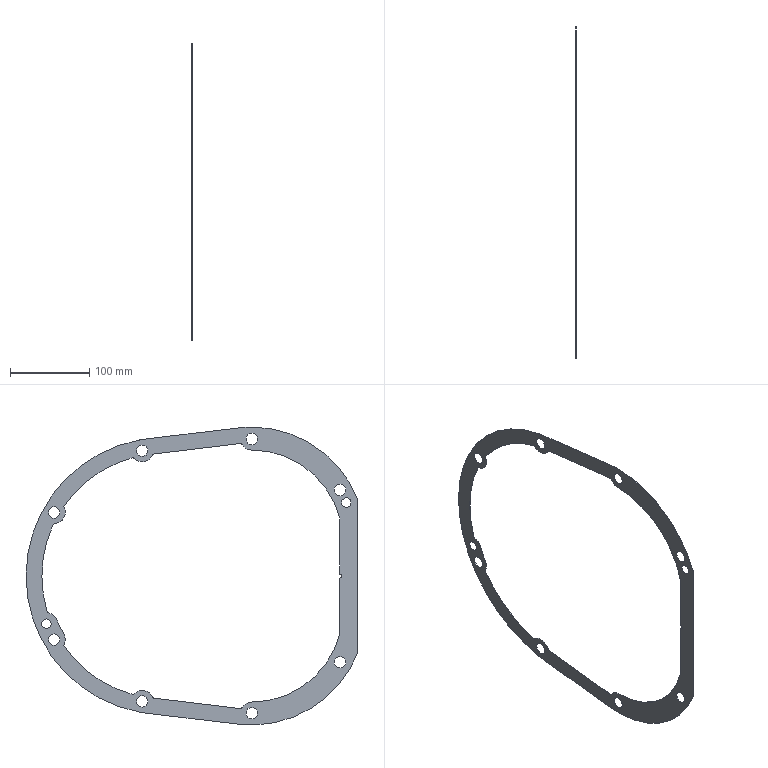Part | STEP file | Input 109 | 1 solid | 69 faces | box 0.5 x 420 x 377 mm | volume 13724 mm3 | cylinder 59 | plane 10 | commonest cylinder face diameters 6 x17 14.5 x16 28 x10 12 x4 288 x3 310 x3